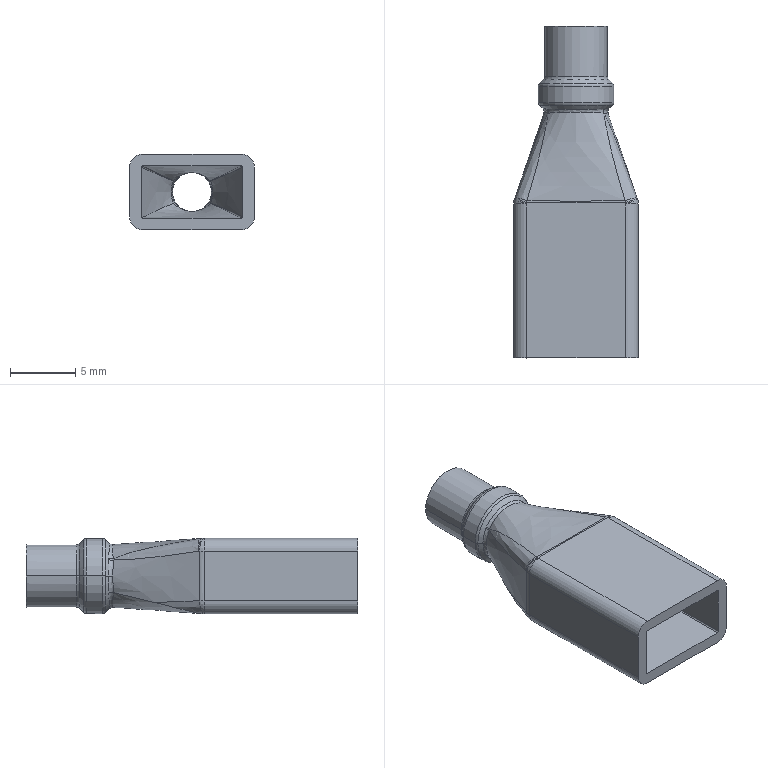Part | STEP file | ZHICHA_1_1_1 | 1 solid | 104 faces | box 9.6 x 25.5 x 5.8 mm | volume 487.442 mm3 | spline 41 | cylinder 22 | sphere 14 | plane 10 | torus 9 | cone 8 | commonest cylinder face diameters 0.2 x7 2 x7 3 x2 4 x2 4.8 x2 5.8 x2